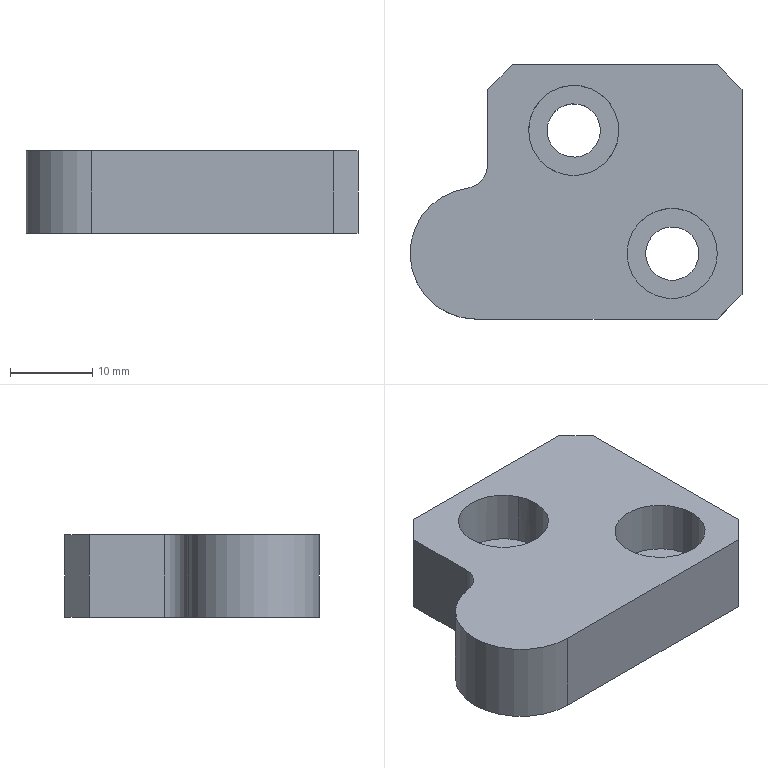Part | STEP file | 1_id1314_x_t | 1 solid | 24 faces | box 40.468 x 31 x 10 mm | volume 8665 mm3 | cylinder 12 | plane 12 | commonest cylinder face diameters 6.5 x4 11 x4 12 x2 6 x1 16 x1